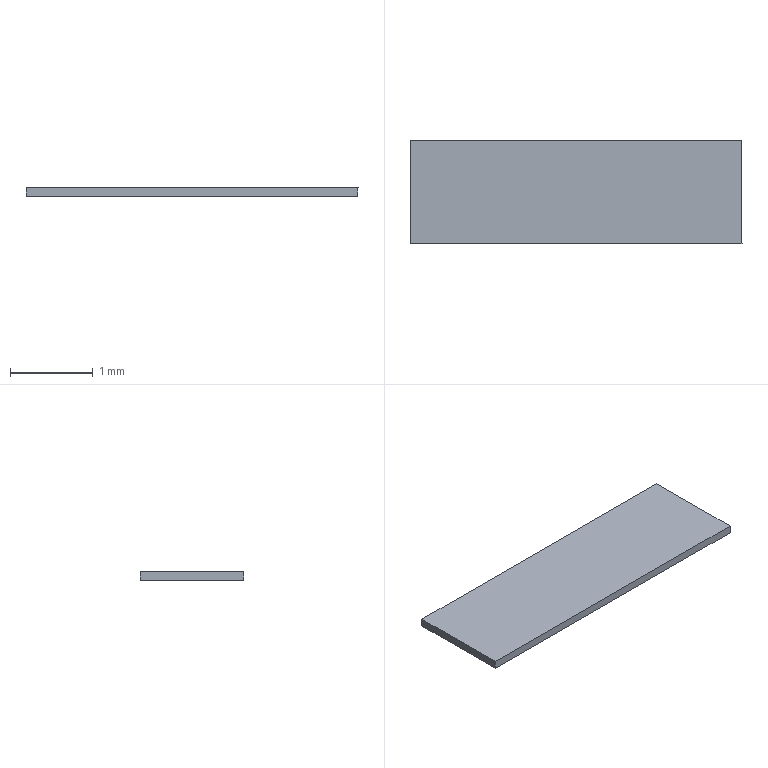Part | STEP file | RJ-USIO-V1_2-220411_345 | 1 solid | 6 faces | box 4 x 1.25 x 0.1 mm | volume 0.5 mm3 | plane 6
STEP:
#1=CARTESIAN_POINT('',(0.,0.,0.));
#2=DIRECTION('',(0.,0.,1.));
#3=DIRECTION('',(1.,0.,0.));
#4=AXIS2_PLACEMENT_3D('',#1,#2,#3);
#5=CARTESIAN_POINT('',(73.9,25.85,0.000000087));
#6=VERTEX_POINT('',#5);
#7=CARTESIAN_POINT('',(77.9,25.85,-0.000000087));
#8=VERTEX_POINT('',#7);
#9=CARTESIAN_POINT('',(73.9,25.85,0.000000087));
#10=DIRECTION('',(1.,0.000000044,-0.000000044));
#11=VECTOR('',#10,1.);
#12=LINE('',#9,#11);
#13=CARTESIAN_POINT('',(73.9,25.85,0.000000087));
#14=DIRECTION('',(0.000000044,0.,1.));
#15=DIRECTION('',(-1.,-0.000000044,0.000000044));
#16=AXIS2_PLACEMENT_3D('',#13,#14,#15);
#17=PLANE('',#16);
#18=CARTESIAN_POINT('',(0.,0.));
#19=DIRECTION('',(-1.,0.));
#20=VECTOR('',#19,1.);
#21=LINE('',#18,#20);
#22=(GEOMETRIC_REPRESENTATION_CONTEXT(2)PARAMETRIC_REPRESENTATION_CONTEXT()REPRESENTATION_CONTEXT('',''));
#23=DEFINITIONAL_REPRESENTATION('',(#21),#22);
#24=PCURVE('',#17,#23);
#25=CARTESIAN_POINT('',(77.9,25.85,0.1));
#26=DIRECTION('',(0.000000044,-1.,0.));
#27=DIRECTION('',(-1.,-0.000000044,0.000000044));
#28=AXIS2_PLACEMENT_3D('',#25,#26,#27);
#29=PLANE('',#28);
#30=CARTESIAN_POINT('',(4.,0.1));
#31=DIRECTION('',(-1.,0.));
#32=VECTOR('',#31,1.);
#33=LINE('',#30,#32);
#34=(GEOMETRIC_REPRESENTATION_CONTEXT(2)PARAMETRIC_REPRESENTATION_CONTEXT()REPRESENTATION_CONTEXT('',''));
#35=DEFINITIONAL_REPRESENTATION('',(#33),#34);
#36=PCURVE('',#29,#35);
#37=SURFACE_CURVE('',#12,(#24,#36),.PCURVE_S1.);
#38=EDGE_CURVE('',#6,#8,#37,.T.);
#39=ORIENTED_EDGE('',*,*,#38,.F.);
#40=CARTESIAN_POINT('',(73.9,24.6,0.000000087));
#41=VERTEX_POINT('',#40);
#42=CARTESIAN_POINT('',(73.9,24.6,0.000000087));
#43=DIRECTION('',(-0.000000044,1.,0.));
#44=VECTOR('',#43,1.);
#45=LINE('',#42,#44);
#46=CARTESIAN_POINT('',(0.,1.25));
#47=DIRECTION('',(0.,-1.));
#48=VECTOR('',#47,1.);
#49=LINE('',#46,#48);
#50=(GEOMETRIC_REPRESENTATION_CONTEXT(2)PARAMETRIC_REPRESENTATION_CONTEXT()REPRESENTATION_CONTEXT('',''));
#51=DEFINITIONAL_REPRESENTATION('',(#49),#50);
#52=PCURVE('',#17,#51);
#53=CARTESIAN_POINT('',(73.9,25.85,0.1));
#54=DIRECTION('',(1.,0.000000044,-0.000000044));
#55=DIRECTION('',(0.000000044,-1.,0.));
#56=AXIS2_PLACEMENT_3D('',#53,#54,#55);
#57=PLANE('',#56);
#58=CARTESIAN_POINT('',(1.25,0.1));
#59=DIRECTION('',(-1.,0.));
#60=VECTOR('',#59,1.);
#61=LINE('',#58,#60);
#62=(GEOMETRIC_REPRESENTATION_CONTEXT(2)PARAMETRIC_REPRESENTATION_CONTEXT()REPRESENTATION_CONTEXT('',''));
#63=DEFINITIONAL_REPRESENTATION('',(#61),#62);
#64=PCURVE('',#57,#63);
#65=SURFACE_CURVE('',#45,(#52,#64),.PCURVE_S1.);
#66=EDGE_CURVE('',#41,#6,#65,.T.);
#67=ORIENTED_EDGE('',*,*,#66,.F.);
#68=CARTESIAN_POINT('',(77.9,24.6,-0.000000087));
#69=VERTEX_POINT('',#68);
#70=CARTESIAN_POINT('',(77.9,24.6,-0.000000087));
#71=DIRECTION('',(-1.,-0.000000044,0.000000044));
#72=VECTOR('',#71,1.);
#73=LINE('',#70,#72);
#74=CARTESIAN_POINT('',(-4.,1.25));
#75=DIRECTION('',(1.,0.));
#76=VECTOR('',#75,1.);
#77=LINE('',#74,#76);
#78=(GEOMETRIC_REPRESENTATION_CONTEXT(2)PARAMETRIC_REPRESENTATION_CONTEXT()REPRESENTATION_CONTEXT('',''));
#79=DEFINITIONAL_REPRESENTATION('',(#77),#78);
#80=PCURVE('',#17,#79);
#81=CARTESIAN_POINT('',(77.9,24.6,0.1));
#82=DIRECTION('',(-0.000000044,1.,0.));
#83=DIRECTION('',(1.,0.000000044,-0.000000044));
#84=AXIS2_PLACEMENT_3D('',#81,#82,#83);
#85=PLANE('',#84);
#86=CARTESIAN_POINT('',(0.,0.1));
#87=DIRECTION('',(-1.,0.));
#88=VECTOR('',#87,1.);
#89=LINE('',#86,#88);
#90=(GEOMETRIC_REPRESENTATION_CONTEXT(2)PARAMETRIC_REPRESENTATION_CONTEXT()REPRESENTATION_CONTEXT('',''));
#91=DEFINITIONAL_REPRESENTATION('',(#89),#90);
#92=PCURVE('',#85,#91);
#93=SURFACE_CURVE('',#73,(#80,#92),.PCURVE_S1.);
#94=EDGE_CURVE('',#69,#41,#93,.T.);
#95=ORIENTED_EDGE('',*,*,#94,.F.);
#96=CARTESIAN_POINT('',(77.9,25.85,-0.000000087));
#97=DIRECTION('',(0.000000044,-1.,0.));
#98=VECTOR('',#97,1.);
#99=LINE('',#96,#98);
#100=CARTESIAN_POINT('',(-4.,0.));
#101=DIRECTION('',(0.,1.));
#102=VECTOR('',#101,1.);
#103=LINE('',#100,#102);
#104=(GEOMETRIC_REPRESENTATION_CONTEXT(2)PARAMETRIC_REPRESENTATION_CONTEXT()REPRESENTATION_CONTEXT('',''));
#105=DEFINITIONAL_REPRESENTATION('',(#103),#104);
#106=PCURVE('',#17,#105);
#107=CARTESIAN_POINT('',(77.9,25.85,0.1));
#108=DIRECTION('',(-1.,-0.000000044,0.000000044));
#109=DIRECTION('',(-0.000000044,1.,0.));
#110=AXIS2_PLACEMENT_3D('',#107,#108,#109);
#111=PLANE('',#110);
#112=CARTESIAN_POINT('',(0.,0.1));
#113=DIRECTION('',(-1.,0.));
#114=VECTOR('',#113,1.);
#115=LINE('',#112,#114);
#116=(GEOMETRIC_REPRESENTATION_CONTEXT(2)PARAMETRIC_REPRESENTATION_CONTEXT()REPRESENTATION_CONTEXT('',''));
#117=DEFINITIONAL_REPRESENTATION('',(#115),#116);
#118=PCURVE('',#111,#117);
#119=SURFACE_CURVE('',#99,(#106,#118),.PCURVE_S1.);
#120=EDGE_CURVE('',#8,#69,#119,.T.);
#121=ORIENTED_EDGE('',*,*,#120,.F.);
#122=EDGE_LOOP('',(#39,#67,#95,#121));
#123=FACE_BOUND('',#122,.F.);
#124=ADVANCED_FACE('',(#123),#17,.F.);
#125=ORIENTED_EDGE('',*,*,#38,.T.);
#126=CARTESIAN_POINT('',(77.9,25.85,0.1));
#127=VERTEX_POINT('',#126);
#128=CARTESIAN_POINT('',(77.9,25.85,-0.000000087));
#129=DIRECTION('',(0.000000044,0.,1.));
#130=VECTOR('',#129,1.);
#131=LINE('',#128,#130);
#132=CARTESIAN_POINT('',(0.,0.1));
#133=DIRECTION('',(0.,-1.));
#134=VECTOR('',#133,1.);
#135=LINE('',#132,#134);
#136=(GEOMETRIC_REPRESENTATION_CONTEXT(2)PARAMETRIC_REPRESENTATION_CONTEXT()REPRESENTATION_CONTEXT('',''));
#137=DEFINITIONAL_REPRESENTATION('',(#135),#136);
#138=PCURVE('',#29,#137);
#139=CARTESIAN_POINT('',(0.,0.1));
#140=DIRECTION('',(0.,-1.));
#141=VECTOR('',#140,1.);
#142=LINE('',#139,#141);
#143=(GEOMETRIC_REPRESENTATION_CONTEXT(2)PARAMETRIC_REPRESENTATION_CONTEXT()REPRESENTATION_CONTEXT('',''));
#144=DEFINITIONAL_REPRESENTATION('',(#142),#143);
#145=PCURVE('',#111,#144);
#146=SURFACE_CURVE('',#131,(#138,#145),.PCURVE_S1.);
#147=EDGE_CURVE('',#8,#127,#146,.T.);
#148=ORIENTED_EDGE('',*,*,#147,.T.);
#149=CARTESIAN_POINT('',(73.9,25.85,0.1));
#150=VERTEX_POINT('',#149);
#151=CARTESIAN_POINT('',(73.9,25.85,0.1));
#152=DIRECTION('',(1.,0.000000044,-0.000000044));
#153=VECTOR('',#152,1.);
#154=LINE('',#151,#153);
#155=CARTESIAN_POINT('',(4.,0.));
#156=DIRECTION('',(-1.,0.));
#157=VECTOR('',#156,1.);
#158=LINE('',#155,#157);
#159=(GEOMETRIC_REPRESENTATION_CONTEXT(2)PARAMETRIC_REPRESENTATION_CONTEXT()REPRESENTATION_CONTEXT('',''));
#160=DEFINITIONAL_REPRESENTATION('',(#158),#159);
#161=PCURVE('',#29,#160);
#162=CARTESIAN_POINT('',(73.9,25.85,0.1));
#163=DIRECTION('',(0.000000044,0.,1.));
#164=DIRECTION('',(-1.,-0.000000044,0.000000044));
#165=AXIS2_PLACEMENT_3D('',#162,#163,#164);
#166=PLANE('',#165);
#167=CARTESIAN_POINT('',(0.,0.));
#168=DIRECTION('',(-1.,0.));
#169=VECTOR('',#168,1.);
#170=LINE('',#167,#169);
#171=(GEOMETRIC_REPRESENTATION_CONTEXT(2)PARAMETRIC_REPRESENTATION_CONTEXT()REPRESENTATION_CONTEXT('',''));
#172=DEFINITIONAL_REPRESENTATION('',(#170),#171);
#173=PCURVE('',#166,#172);
#174=SURFACE_CURVE('',#154,(#161,#173),.PCURVE_S1.);
#175=EDGE_CURVE('',#150,#127,#174,.T.);
#176=ORIENTED_EDGE('',*,*,#175,.F.);
#177=CARTESIAN_POINT('',(73.9,25.85,0.000000087));
#178=DIRECTION('',(0.000000044,0.,1.));
#179=VECTOR('',#178,1.);
#180=LINE('',#177,#179);
#181=CARTESIAN_POINT('',(4.,0.1));
#182=DIRECTION('',(0.,-1.));
#183=VECTOR('',#182,1.);
#184=LINE('',#181,#183);
#185=(GEOMETRIC_REPRESENTATION_CONTEXT(2)PARAMETRIC_REPRESENTATION_CONTEXT()REPRESENTATION_CONTEXT('',''));
#186=DEFINITIONAL_REPRESENTATION('',(#184),#185);
#187=PCURVE('',#29,#186);
#188=CARTESIAN_POINT('',(0.,0.1));
#189=DIRECTION('',(0.,-1.));
#190=VECTOR('',#189,1.);
#191=LINE('',#188,#190);
#192=(GEOMETRIC_REPRESENTATION_CONTEXT(2)PARAMETRIC_REPRESENTATION_CONTEXT()REPRESENTATION_CONTEXT('',''));
#193=DEFINITIONAL_REPRESENTATION('',(#191),#192);
#194=PCURVE('',#57,#193);
#195=SURFACE_CURVE('',#180,(#187,#194),.PCURVE_S1.);
#196=EDGE_CURVE('',#6,#150,#195,.T.);
#197=ORIENTED_EDGE('',*,*,#196,.F.);
#198=EDGE_LOOP('',(#125,#148,#176,#197));
#199=FACE_BOUND('',#198,.F.);
#200=ADVANCED_FACE('',(#199),#29,.F.);
#201=ORIENTED_EDGE('',*,*,#120,.T.);
#202=CARTESIAN_POINT('',(77.9,24.6,0.1));
#203=VERTEX_POINT('',#202);
#204=CARTESIAN_POINT('',(77.9,24.6,-0.000000087));
#205=DIRECTION('',(0.000000044,0.,1.));
#206=VECTOR('',#205,1.);
#207=LINE('',#204,#206);
#208=CARTESIAN_POINT('',(-1.25,0.1));
#209=DIRECTION('',(0.,-1.));
#210=VECTOR('',#209,1.);
#211=LINE('',#208,#210);
#212=(GEOMETRIC_REPRESENTATION_CONTEXT(2)PARAMETRIC_REPRESENTATION_CONTEXT()REPRESENTATION_CONTEXT('',''));
#213=DEFINITIONAL_REPRESENTATION('',(#211),#212);
#214=PCURVE('',#111,#213);
#215=CARTESIAN_POINT('',(0.,0.1));
#216=DIRECTION('',(0.,-1.));
#217=VECTOR('',#216,1.);
#218=LINE('',#215,#217);
#219=(GEOMETRIC_REPRESENTATION_CONTEXT(2)PARAMETRIC_REPRESENTATION_CONTEXT()REPRESENTATION_CONTEXT('',''));
#220=DEFINITIONAL_REPRESENTATION('',(#218),#219);
#221=PCURVE('',#85,#220);
#222=SURFACE_CURVE('',#207,(#214,#221),.PCURVE_S1.);
#223=EDGE_CURVE('',#69,#203,#222,.T.);
#224=ORIENTED_EDGE('',*,*,#223,.T.);
#225=CARTESIAN_POINT('',(77.9,25.85,0.1));
#226=DIRECTION('',(0.000000044,-1.,0.));
#227=VECTOR('',#226,1.);
#228=LINE('',#225,#227);
#229=CARTESIAN_POINT('',(0.,0.));
#230=DIRECTION('',(-1.,0.));
#231=VECTOR('',#230,1.);
#232=LINE('',#229,#231);
#233=(GEOMETRIC_REPRESENTATION_CONTEXT(2)PARAMETRIC_REPRESENTATION_CONTEXT()REPRESENTATION_CONTEXT('',''));
#234=DEFINITIONAL_REPRESENTATION('',(#232),#233);
#235=PCURVE('',#111,#234);
#236=CARTESIAN_POINT('',(-4.,0.));
#237=DIRECTION('',(0.,1.));
#238=VECTOR('',#237,1.);
#239=LINE('',#236,#238);
#240=(GEOMETRIC_REPRESENTATION_CONTEXT(2)PARAMETRIC_REPRESENTATION_CONTEXT()REPRESENTATION_CONTEXT('',''));
#241=DEFINITIONAL_REPRESENTATION('',(#239),#240);
#242=PCURVE('',#166,#241);
#243=SURFACE_CURVE('',#228,(#235,#242),.PCURVE_S1.);
#244=EDGE_CURVE('',#127,#203,#243,.T.);
#245=ORIENTED_EDGE('',*,*,#244,.F.);
#246=ORIENTED_EDGE('',*,*,#147,.F.);
#247=EDGE_LOOP('',(#201,#224,#245,#246));
#248=FACE_BOUND('',#247,.F.);
#249=ADVANCED_FACE('',(#248),#111,.F.);
#250=ORIENTED_EDGE('',*,*,#94,.T.);
#251=CARTESIAN_POINT('',(73.9,24.6,0.1));
#252=VERTEX_POINT('',#251);
#253=CARTESIAN_POINT('',(73.9,24.6,0.000000087));
#254=DIRECTION('',(0.000000044,0.,1.));
#255=VECTOR('',#254,1.);
#256=LINE('',#253,#255);
#257=CARTESIAN_POINT('',(-4.,0.1));
#258=DIRECTION('',(0.,-1.));
#259=VECTOR('',#258,1.);
#260=LINE('',#257,#259);
#261=(GEOMETRIC_REPRESENTATION_CONTEXT(2)PARAMETRIC_REPRESENTATION_CONTEXT()REPRESENTATION_CONTEXT('',''));
#262=DEFINITIONAL_REPRESENTATION('',(#260),#261);
#263=PCURVE('',#85,#262);
#264=CARTESIAN_POINT('',(1.25,0.1));
#265=DIRECTION('',(0.,-1.));
#266=VECTOR('',#265,1.);
#267=LINE('',#264,#266);
#268=(GEOMETRIC_REPRESENTATION_CONTEXT(2)PARAMETRIC_REPRESENTATION_CONTEXT()REPRESENTATION_CONTEXT('',''));
#269=DEFINITIONAL_REPRESENTATION('',(#267),#268);
#270=PCURVE('',#57,#269);
#271=SURFACE_CURVE('',#256,(#263,#270),.PCURVE_S1.);
#272=EDGE_CURVE('',#41,#252,#271,.T.);
#273=ORIENTED_EDGE('',*,*,#272,.T.);
#274=CARTESIAN_POINT('',(77.9,24.6,0.1));
#275=DIRECTION('',(-1.,-0.000000044,0.000000044));
#276=VECTOR('',#275,1.);
#277=LINE('',#274,#276);
#278=CARTESIAN_POINT('',(0.,0.));
#279=DIRECTION('',(-1.,0.));
#280=VECTOR('',#279,1.);
#281=LINE('',#278,#280);
#282=(GEOMETRIC_REPRESENTATION_CONTEXT(2)PARAMETRIC_REPRESENTATION_CONTEXT()REPRESENTATION_CONTEXT('',''));
#283=DEFINITIONAL_REPRESENTATION('',(#281),#282);
#284=PCURVE('',#85,#283);
#285=CARTESIAN_POINT('',(-4.,1.25));
#286=DIRECTION('',(1.,0.));
#287=VECTOR('',#286,1.);
#288=LINE('',#285,#287);
#289=(GEOMETRIC_REPRESENTATION_CONTEXT(2)PARAMETRIC_REPRESENTATION_CONTEXT()REPRESENTATION_CONTEXT('',''));
#290=DEFINITIONAL_REPRESENTATION('',(#288),#289);
#291=PCURVE('',#166,#290);
#292=SURFACE_CURVE('',#277,(#284,#291),.PCURVE_S1.);
#293=EDGE_CURVE('',#203,#252,#292,.T.);
#294=ORIENTED_EDGE('',*,*,#293,.F.);
#295=ORIENTED_EDGE('',*,*,#223,.F.);
#296=EDGE_LOOP('',(#250,#273,#294,#295));
#297=FACE_BOUND('',#296,.F.);
#298=ADVANCED_FACE('',(#297),#85,.F.);
#299=ORIENTED_EDGE('',*,*,#66,.T.);
#300=ORIENTED_EDGE('',*,*,#196,.T.);
#301=CARTESIAN_POINT('',(73.9,24.6,0.1));
#302=DIRECTION('',(-0.000000044,1.,0.));
#303=VECTOR('',#302,1.);
#304=LINE('',#301,#303);
#305=CARTESIAN_POINT('',(1.25,0.));
#306=DIRECTION('',(-1.,0.));
#307=VECTOR('',#306,1.);
#308=LINE('',#305,#307);
#309=(GEOMETRIC_REPRESENTATION_CONTEXT(2)PARAMETRIC_REPRESENTATION_CONTEXT()REPRESENTATION_CONTEXT('',''));
#310=DEFINITIONAL_REPRESENTATION('',(#308),#309);
#311=PCURVE('',#57,#310);
#312=CARTESIAN_POINT('',(0.,1.25));
#313=DIRECTION('',(0.,-1.));
#314=VECTOR('',#313,1.);
#315=LINE('',#312,#314);
#316=(GEOMETRIC_REPRESENTATION_CONTEXT(2)PARAMETRIC_REPRESENTATION_CONTEXT()REPRESENTATION_CONTEXT('',''));
#317=DEFINITIONAL_REPRESENTATION('',(#315),#316);
#318=PCURVE('',#166,#317);
#319=SURFACE_CURVE('',#304,(#311,#318),.PCURVE_S1.);
#320=EDGE_CURVE('',#252,#150,#319,.T.);
#321=ORIENTED_EDGE('',*,*,#320,.F.);
#322=ORIENTED_EDGE('',*,*,#272,.F.);
#323=EDGE_LOOP('',(#299,#300,#321,#322));
#324=FACE_BOUND('',#323,.F.);
#325=ADVANCED_FACE('',(#324),#57,.F.);
#326=ORIENTED_EDGE('',*,*,#175,.T.);
#327=ORIENTED_EDGE('',*,*,#244,.T.);
#328=ORIENTED_EDGE('',*,*,#293,.T.);
#329=ORIENTED_EDGE('',*,*,#320,.T.);
#330=EDGE_LOOP('',(#326,#327,#328,#329));
#331=FACE_BOUND('',#330,.F.);
#332=ADVANCED_FACE('',(#331),#166,.T.);
#333=CLOSED_SHELL('',(#124,#200,#249,#298,#325,#332));
#334=MANIFOLD_SOLID_BREP('',#333);
#335=(LENGTH_UNIT()NAMED_UNIT(*)SI_UNIT(.MILLI.,.METRE.));
#336=UNCERTAINTY_MEASURE_WITH_UNIT(LENGTH_MEASURE(0.0000001),#335,'','');
#337=(NAMED_UNIT(*)PLANE_ANGLE_UNIT()SI_UNIT($,.RADIAN.));
#338=(NAMED_UNIT(*)SI_UNIT($,.STERADIAN.)SOLID_ANGLE_UNIT());
#339=(GEOMETRIC_REPRESENTATION_CONTEXT(3)GLOBAL_UNCERTAINTY_ASSIGNED_CONTEXT((#336))GLOBAL_UNIT_ASSIGNED_CONTEXT((#335,#337,#338))REPRESENTATION_CONTEXT('',''));
#340=ADVANCED_BREP_SHAPE_REPRESENTATION('',(#4,#334),#339);